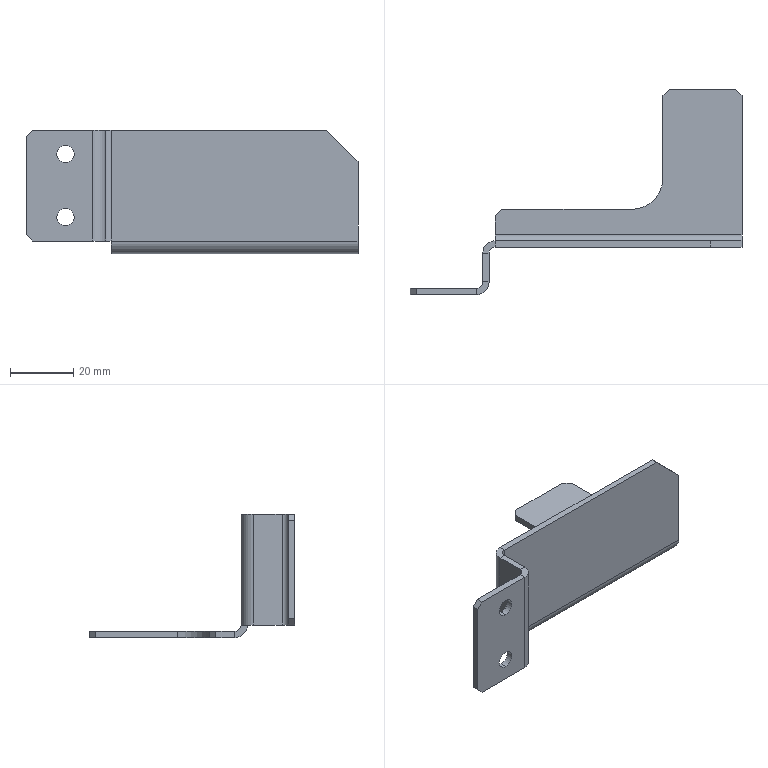Part | NX | features BREP 1 | 1 solid | 43 faces | box 105 x 65 x 39 mm | volume 11931 mm3 | plane 32 | cylinder 11 | commonest cylinder face diameters 5.5 x4 4 x3 8 x3 20 x1
STEP:
#1=CARTESIAN_POINT('',(2.,0.,17.5));
#2=VERTEX_POINT('',#1);
#3=CARTESIAN_POINT('',(0.,0.,15.5));
#4=VERTEX_POINT('',#3);
#5=CARTESIAN_POINT('',(0.,0.,15.5));
#6=DIRECTION('',(-0.7071,0.,-0.7071));
#7=VECTOR('',#6,1000.);
#8=LINE('',#5,#7);
#9=EDGE_CURVE('',#2,#4,#8,.T.);
#10=ORIENTED_EDGE('',*,*,#9,.F.);
#11=CARTESIAN_POINT('',(2.,2.,17.5));
#12=VERTEX_POINT('',#11);
#13=CARTESIAN_POINT('',(2.,4.,17.5));
#14=DIRECTION('',(0.,-1.,0.));
#15=VECTOR('',#14,1000.);
#16=LINE('',#13,#15);
#17=EDGE_CURVE('',#12,#2,#16,.T.);
#18=ORIENTED_EDGE('',*,*,#17,.F.);
#19=CARTESIAN_POINT('',(0.,2.,15.5));
#20=VERTEX_POINT('',#19);
#21=CARTESIAN_POINT('',(1.,2.,16.5));
#22=DIRECTION('',(0.7071,0.,0.7071));
#23=VECTOR('',#22,1000.);
#24=LINE('',#21,#23);
#25=EDGE_CURVE('',#20,#12,#24,.T.);
#26=ORIENTED_EDGE('',*,*,#25,.F.);
#27=CARTESIAN_POINT('',(0.,0.,15.5));
#28=DIRECTION('',(0.,1.,0.));
#29=VECTOR('',#28,1000.);
#30=LINE('',#27,#29);
#31=EDGE_CURVE('',#4,#20,#30,.T.);
#32=ORIENTED_EDGE('',*,*,#31,.F.);
#33=EDGE_LOOP('',(#10,#18,#26,#32));
#34=FACE_BOUND('',#33,.T.);
#35=CARTESIAN_POINT('',(0.,0.,15.5));
#36=DIRECTION('',(0.7071,0.,-0.7071));
#37=DIRECTION('',(0.,1.,0.));
#38=AXIS2_PLACEMENT_3D('',#35,#36,#37);
#39=PLANE('',#38);
#40=ADVANCED_FACE('',(#34),#39,.F.);
#41=CARTESIAN_POINT('',(0.,0.,-15.5));
#42=VERTEX_POINT('',#41);
#43=CARTESIAN_POINT('',(2.,0.,-17.5));
#44=VERTEX_POINT('',#43);
#45=CARTESIAN_POINT('',(2.,0.,-17.5));
#46=DIRECTION('',(0.7071,0.,-0.7071));
#47=VECTOR('',#46,1000.);
#48=LINE('',#45,#47);
#49=EDGE_CURVE('',#42,#44,#48,.T.);
#50=ORIENTED_EDGE('',*,*,#49,.F.);
#51=CARTESIAN_POINT('',(0.,2.,-15.5));
#52=VERTEX_POINT('',#51);
#53=CARTESIAN_POINT('',(0.,0.,-15.5));
#54=DIRECTION('',(0.,-1.,0.));
#55=VECTOR('',#54,1000.);
#56=LINE('',#53,#55);
#57=EDGE_CURVE('',#52,#42,#56,.T.);
#58=ORIENTED_EDGE('',*,*,#57,.F.);
#59=CARTESIAN_POINT('',(2.,2.,-17.5));
#60=VERTEX_POINT('',#59);
#61=CARTESIAN_POINT('',(-16.5,2.,1.));
#62=DIRECTION('',(-0.7071,0.,0.7071));
#63=VECTOR('',#62,1000.);
#64=LINE('',#61,#63);
#65=EDGE_CURVE('',#60,#52,#64,.T.);
#66=ORIENTED_EDGE('',*,*,#65,.F.);
#67=CARTESIAN_POINT('',(2.,2.,-17.5));
#68=DIRECTION('',(0.,1.,0.));
#69=VECTOR('',#68,1000.);
#70=LINE('',#67,#69);
#71=EDGE_CURVE('',#44,#60,#70,.T.);
#72=ORIENTED_EDGE('',*,*,#71,.F.);
#73=EDGE_LOOP('',(#50,#58,#66,#72));
#74=FACE_BOUND('',#73,.T.);
#75=CARTESIAN_POINT('',(2.,13.,-17.5));
#76=DIRECTION('',(-0.7071,0.,-0.7071));
#77=DIRECTION('',(0.,-1.,0.));
#78=AXIS2_PLACEMENT_3D('',#75,#76,#77);
#79=PLANE('',#78);
#80=ADVANCED_FACE('',(#74),#79,.T.);
#81=CARTESIAN_POINT('',(29.,27.,-19.5));
#82=VERTEX_POINT('',#81);
#83=CARTESIAN_POINT('',(27.,25.,-19.5));
#84=VERTEX_POINT('',#83);
#85=CARTESIAN_POINT('',(27.,25.,-19.5));
#86=DIRECTION('',(-0.7071,-0.7071,0.));
#87=VECTOR('',#86,1000.);
#88=LINE('',#85,#87);
#89=EDGE_CURVE('',#82,#84,#88,.T.);
#90=ORIENTED_EDGE('',*,*,#89,.F.);
#91=CARTESIAN_POINT('',(29.,27.,-21.5));
#92=VERTEX_POINT('',#91);
#93=CARTESIAN_POINT('',(29.,27.,-19.5));
#94=DIRECTION('',(0.,0.,1.));
#95=VECTOR('',#94,1000.);
#96=LINE('',#93,#95);
#97=EDGE_CURVE('',#92,#82,#96,.T.);
#98=ORIENTED_EDGE('',*,*,#97,.F.);
#99=CARTESIAN_POINT('',(27.,25.,-21.5));
#100=VERTEX_POINT('',#99);
#101=CARTESIAN_POINT('',(1.,-1.,-21.5));
#102=DIRECTION('',(0.7071,0.7071,0.));
#103=VECTOR('',#102,1000.);
#104=LINE('',#101,#103);
#105=EDGE_CURVE('',#100,#92,#104,.T.);
#106=ORIENTED_EDGE('',*,*,#105,.F.);
#107=CARTESIAN_POINT('',(27.,25.,-21.5));
#108=DIRECTION('',(0.,0.,-1.));
#109=VECTOR('',#108,1000.);
#110=LINE('',#107,#109);
#111=EDGE_CURVE('',#84,#100,#110,.T.);
#112=ORIENTED_EDGE('',*,*,#111,.F.);
#113=EDGE_LOOP('',(#90,#98,#106,#112));
#114=FACE_BOUND('',#113,.T.);
#115=CARTESIAN_POINT('',(27.,25.,-21.5));
#116=DIRECTION('',(-0.7071,0.7071,0.));
#117=DIRECTION('',(0.,0.,1.));
#118=AXIS2_PLACEMENT_3D('',#115,#116,#117);
#119=PLANE('',#118);
#120=ADVANCED_FACE('',(#114),#119,.T.);
#121=CARTESIAN_POINT('',(82.,65.,-19.5));
#122=VERTEX_POINT('',#121);
#123=CARTESIAN_POINT('',(80.,63.,-19.5));
#124=VERTEX_POINT('',#123);
#125=CARTESIAN_POINT('',(80.,63.,-19.5));
#126=DIRECTION('',(-0.7071,-0.7071,0.));
#127=VECTOR('',#126,1000.);
#128=LINE('',#125,#127);
#129=EDGE_CURVE('',#122,#124,#128,.T.);
#130=ORIENTED_EDGE('',*,*,#129,.F.);
#131=CARTESIAN_POINT('',(82.,65.,-21.5));
#132=VERTEX_POINT('',#131);
#133=CARTESIAN_POINT('',(82.,65.,-19.5));
#134=DIRECTION('',(0.,0.,1.));
#135=VECTOR('',#134,1000.);
#136=LINE('',#133,#135);
#137=EDGE_CURVE('',#132,#122,#136,.T.);
#138=ORIENTED_EDGE('',*,*,#137,.F.);
#139=CARTESIAN_POINT('',(80.,63.,-21.5));
#140=VERTEX_POINT('',#139);
#141=CARTESIAN_POINT('',(8.5,-8.5,-21.5));
#142=DIRECTION('',(0.7071,0.7071,0.));
#143=VECTOR('',#142,1000.);
#144=LINE('',#141,#143);
#145=EDGE_CURVE('',#140,#132,#144,.T.);
#146=ORIENTED_EDGE('',*,*,#145,.F.);
#147=CARTESIAN_POINT('',(80.,63.,-21.5));
#148=DIRECTION('',(0.,0.,-1.));
#149=VECTOR('',#148,1000.);
#150=LINE('',#147,#149);
#151=EDGE_CURVE('',#124,#140,#150,.T.);
#152=ORIENTED_EDGE('',*,*,#151,.F.);
#153=EDGE_LOOP('',(#130,#138,#146,#152));
#154=FACE_BOUND('',#153,.T.);
#155=CARTESIAN_POINT('',(80.,63.,17.5));
#156=DIRECTION('',(-0.7071,0.7071,0.));
#157=DIRECTION('',(0.,0.,1.));
#158=AXIS2_PLACEMENT_3D('',#155,#156,#157);
#159=PLANE('',#158);
#160=ADVANCED_FACE('',(#154),#159,.T.);
#161=CARTESIAN_POINT('',(103.,65.,-21.5));
#162=VERTEX_POINT('',#161);
#163=CARTESIAN_POINT('',(105.,63.,-21.5));
#164=VERTEX_POINT('',#163);
#165=CARTESIAN_POINT('',(84.,84.,-21.5));
#166=DIRECTION('',(0.7071,-0.7071,0.));
#167=VECTOR('',#166,1000.);
#168=LINE('',#165,#167);
#169=EDGE_CURVE('',#162,#164,#168,.T.);
#170=ORIENTED_EDGE('',*,*,#169,.F.);
#171=CARTESIAN_POINT('',(103.,65.,-19.5));
#172=VERTEX_POINT('',#171);
#173=CARTESIAN_POINT('',(103.,65.,-21.5));
#174=DIRECTION('',(0.,0.,-1.));
#175=VECTOR('',#174,1000.);
#176=LINE('',#173,#175);
#177=EDGE_CURVE('',#172,#162,#176,.T.);
#178=ORIENTED_EDGE('',*,*,#177,.F.);
#179=CARTESIAN_POINT('',(105.,63.,-19.5));
#180=VERTEX_POINT('',#179);
#181=CARTESIAN_POINT('',(105.,63.,-19.5));
#182=DIRECTION('',(-0.7071,0.7071,0.));
#183=VECTOR('',#182,1000.);
#184=LINE('',#181,#183);
#185=EDGE_CURVE('',#180,#172,#184,.T.);
#186=ORIENTED_EDGE('',*,*,#185,.F.);
#187=CARTESIAN_POINT('',(105.,63.,-21.5));
#188=DIRECTION('',(0.,0.,1.));
#189=VECTOR('',#188,1000.);
#190=LINE('',#187,#189);
#191=EDGE_CURVE('',#164,#180,#190,.T.);
#192=ORIENTED_EDGE('',*,*,#191,.F.);
#193=EDGE_LOOP('',(#170,#178,#186,#192));
#194=FACE_BOUND('',#193,.T.);
#195=CARTESIAN_POINT('',(105.,63.,-21.5));
#196=DIRECTION('',(-0.7071,-0.7071,0.));
#197=DIRECTION('',(0.,0.,1.));
#198=AXIS2_PLACEMENT_3D('',#195,#196,#197);
#199=PLANE('',#198);
#200=ADVANCED_FACE('',(#194),#199,.F.);
#201=CARTESIAN_POINT('',(80.,37.,-19.5));
#202=VERTEX_POINT('',#201);
#203=CARTESIAN_POINT('',(70.,27.,-19.5));
#204=VERTEX_POINT('',#203);
#205=CARTESIAN_POINT('',(70.,37.,-19.5));
#206=DIRECTION('',(0.,0.,-1.));
#207=DIRECTION('',(-1.,0.,0.));
#208=AXIS2_PLACEMENT_3D('',#205,#206,#207);
#209=CIRCLE('',#208,10.);
#210=EDGE_CURVE('',#202,#204,#209,.T.);
#211=ORIENTED_EDGE('',*,*,#210,.F.);
#212=CARTESIAN_POINT('',(80.,37.,-21.5));
#213=VERTEX_POINT('',#212);
#214=CARTESIAN_POINT('',(80.,37.,-19.5));
#215=DIRECTION('',(0.,0.,1.));
#216=VECTOR('',#215,1000.);
#217=LINE('',#214,#216);
#218=EDGE_CURVE('',#213,#202,#217,.T.);
#219=ORIENTED_EDGE('',*,*,#218,.F.);
#220=CARTESIAN_POINT('',(70.,27.,-21.5));
#221=VERTEX_POINT('',#220);
#222=CARTESIAN_POINT('',(70.,37.,-21.5));
#223=DIRECTION('',(0.,0.,1.));
#224=DIRECTION('',(-1.,0.,0.));
#225=AXIS2_PLACEMENT_3D('',#222,#223,#224);
#226=CIRCLE('',#225,10.);
#227=EDGE_CURVE('',#221,#213,#226,.T.);
#228=ORIENTED_EDGE('',*,*,#227,.F.);
#229=CARTESIAN_POINT('',(70.,27.,-21.5));
#230=DIRECTION('',(0.,0.,-1.));
#231=VECTOR('',#230,1000.);
#232=LINE('',#229,#231);
#233=EDGE_CURVE('',#204,#221,#232,.T.);
#234=ORIENTED_EDGE('',*,*,#233,.F.);
#235=EDGE_LOOP('',(#211,#219,#228,#234));
#236=FACE_BOUND('',#235,.T.);
#237=CARTESIAN_POINT('',(70.,37.,17.5));
#238=DIRECTION('',(0.,0.,1.));
#239=DIRECTION('',(1.,0.,0.));
#240=AXIS2_PLACEMENT_3D('',#237,#238,#239);
#241=CYLINDRICAL_SURFACE('',#240,10.);
#242=ADVANCED_FACE('',(#236),#241,.F.);
#243=CARTESIAN_POINT('',(95.,17.,17.5));
#244=VERTEX_POINT('',#243);
#245=CARTESIAN_POINT('',(105.,17.,7.5));
#246=VERTEX_POINT('',#245);
#247=CARTESIAN_POINT('',(60.,17.,52.5));
#248=DIRECTION('',(0.7071,0.,-0.7071));
#249=VECTOR('',#248,1000.);
#250=LINE('',#247,#249);
#251=EDGE_CURVE('',#244,#246,#250,.T.);
#252=ORIENTED_EDGE('',*,*,#251,.F.);
#253=CARTESIAN_POINT('',(95.,15.,17.5));
#254=VERTEX_POINT('',#253);
#255=CARTESIAN_POINT('',(95.,13.,17.5));
#256=DIRECTION('',(0.,1.,0.));
#257=VECTOR('',#256,1000.);
#258=LINE('',#255,#257);
#259=EDGE_CURVE('',#254,#244,#258,.T.);
#260=ORIENTED_EDGE('',*,*,#259,.F.);
#261=CARTESIAN_POINT('',(105.,15.,7.5));
#262=VERTEX_POINT('',#261);
#263=CARTESIAN_POINT('',(105.,15.,7.5));
#264=DIRECTION('',(-0.7071,0.,0.7071));
#265=VECTOR('',#264,1000.);
#266=LINE('',#263,#265);
#267=EDGE_CURVE('',#262,#254,#266,.T.);
#268=ORIENTED_EDGE('',*,*,#267,.F.);
#269=CARTESIAN_POINT('',(105.,17.,7.5));
#270=DIRECTION('',(0.,-1.,0.));
#271=VECTOR('',#270,1000.);
#272=LINE('',#269,#271);
#273=EDGE_CURVE('',#246,#262,#272,.T.);
#274=ORIENTED_EDGE('',*,*,#273,.F.);
#275=EDGE_LOOP('',(#252,#260,#268,#274));
#276=FACE_BOUND('',#275,.T.);
#277=CARTESIAN_POINT('',(105.,17.,7.5));
#278=DIRECTION('',(-0.7071,0.,-0.7071));
#279=DIRECTION('',(0.,-1.,0.));
#280=AXIS2_PLACEMENT_3D('',#277,#278,#279);
#281=PLANE('',#280);
#282=ADVANCED_FACE('',(#276),#281,.F.);
#283=CARTESIAN_POINT('',(12.5,2.,-12.75));
#284=VERTEX_POINT('',#283);
#285=CARTESIAN_POINT('',(12.5,0.,-12.75));
#286=VERTEX_POINT('',#285);
#287=CARTESIAN_POINT('',(12.5,2.,-12.75));
#288=DIRECTION('',(0.,1.,0.));
#289=VECTOR('',#288,1000.);
#290=LINE('',#287,#289);
#291=EDGE_CURVE('',#284,#286,#290,.F.);
#292=ORIENTED_EDGE('',*,*,#291,.T.);
#293=CARTESIAN_POINT('',(12.5,0.,-7.25));
#294=VERTEX_POINT('',#293);
#295=CARTESIAN_POINT('',(12.5,0.,-10.));
#296=DIRECTION('',(0.,1.,0.));
#297=DIRECTION('',(0.,0.,1.));
#298=AXIS2_PLACEMENT_3D('',#295,#296,#297);
#299=CIRCLE('',#298,2.75);
#300=EDGE_CURVE('',#294,#286,#299,.T.);
#301=ORIENTED_EDGE('',*,*,#300,.F.);
#302=CARTESIAN_POINT('',(12.5,2.,-7.25));
#303=VERTEX_POINT('',#302);
#304=CARTESIAN_POINT('',(12.5,2.,-7.25));
#305=DIRECTION('',(0.,1.,0.));
#306=VECTOR('',#305,1000.);
#307=LINE('',#304,#306);
#308=EDGE_CURVE('',#303,#294,#307,.F.);
#309=ORIENTED_EDGE('',*,*,#308,.F.);
#310=CARTESIAN_POINT('',(12.5,2.,-10.));
#311=DIRECTION('',(0.,1.,0.));
#312=DIRECTION('',(0.,0.,1.));
#313=AXIS2_PLACEMENT_3D('',#310,#311,#312);
#314=CIRCLE('',#313,2.75);
#315=EDGE_CURVE('',#303,#284,#314,.T.);
#316=ORIENTED_EDGE('',*,*,#315,.T.);
#317=EDGE_LOOP('',(#292,#301,#309,#316));
#318=FACE_BOUND('',#317,.T.);
#319=CARTESIAN_POINT('',(12.5,2.,-10.));
#320=DIRECTION('',(0.,1.,0.));
#321=DIRECTION('',(0.,0.,1.));
#322=AXIS2_PLACEMENT_3D('',#319,#320,#321);
#323=CYLINDRICAL_SURFACE('',#322,2.75);
#324=ADVANCED_FACE('',(#318),#323,.F.);
#325=CARTESIAN_POINT('',(12.5,2.,7.25));
#326=VERTEX_POINT('',#325);
#327=CARTESIAN_POINT('',(12.5,0.,7.25));
#328=VERTEX_POINT('',#327);
#329=CARTESIAN_POINT('',(12.5,2.,7.25));
#330=DIRECTION('',(0.,1.,0.));
#331=VECTOR('',#330,1000.);
#332=LINE('',#329,#331);
#333=EDGE_CURVE('',#326,#328,#332,.F.);
#334=ORIENTED_EDGE('',*,*,#333,.T.);
#335=CARTESIAN_POINT('',(12.5,0.,12.75));
#336=VERTEX_POINT('',#335);
#337=CARTESIAN_POINT('',(12.5,0.,10.));
#338=DIRECTION('',(0.,1.,0.));
#339=DIRECTION('',(0.,0.,1.));
#340=AXIS2_PLACEMENT_3D('',#337,#338,#339);
#341=CIRCLE('',#340,2.75);
#342=EDGE_CURVE('',#336,#328,#341,.T.);
#343=ORIENTED_EDGE('',*,*,#342,.F.);
#344=CARTESIAN_POINT('',(12.5,2.,12.75));
#345=VERTEX_POINT('',#344);
#346=CARTESIAN_POINT('',(12.5,2.,12.75));
#347=DIRECTION('',(0.,1.,0.));
#348=VECTOR('',#347,1000.);
#349=LINE('',#346,#348);
#350=EDGE_CURVE('',#345,#336,#349,.F.);
#351=ORIENTED_EDGE('',*,*,#350,.F.);
#352=CARTESIAN_POINT('',(12.5,2.,10.));
#353=DIRECTION('',(0.,1.,0.));
#354=DIRECTION('',(0.,0.,1.));
#355=AXIS2_PLACEMENT_3D('',#352,#353,#354);
#356=CIRCLE('',#355,2.75);
#357=EDGE_CURVE('',#345,#326,#356,.T.);
#358=ORIENTED_EDGE('',*,*,#357,.T.);
#359=EDGE_LOOP('',(#334,#343,#351,#358));
#360=FACE_BOUND('',#359,.T.);
#361=CARTESIAN_POINT('',(12.5,2.,10.));
#362=DIRECTION('',(0.,1.,0.));
#363=DIRECTION('',(0.,0.,1.));
#364=AXIS2_PLACEMENT_3D('',#361,#362,#363);
#365=CYLINDRICAL_SURFACE('',#364,2.75);
#366=ADVANCED_FACE('',(#360),#365,.F.);
#367=CARTESIAN_POINT('',(80.,0.,-19.5));
#368=DIRECTION('',(0.,-1.,0.));
#369=VECTOR('',#368,1000.);
#370=LINE('',#367,#369);
#371=EDGE_CURVE('',#124,#202,#370,.T.);
#372=ORIENTED_EDGE('',*,*,#371,.F.);
#373=ORIENTED_EDGE('',*,*,#151,.T.);
#374=CARTESIAN_POINT('',(80.,65.,-21.5));
#375=DIRECTION('',(0.,-1.,0.));
#376=VECTOR('',#375,1000.);
#377=LINE('',#374,#376);
#378=EDGE_CURVE('',#140,#213,#377,.T.);
#379=ORIENTED_EDGE('',*,*,#378,.T.);
#380=ORIENTED_EDGE('',*,*,#218,.T.);
#381=EDGE_LOOP('',(#372,#373,#379,#380));
#382=FACE_BOUND('',#381,.T.);
#383=CARTESIAN_POINT('',(80.,65.,17.5));
#384=DIRECTION('',(1.,0.,0.));
#385=DIRECTION('',(0.,0.,-1.));
#386=AXIS2_PLACEMENT_3D('',#383,#384,#385);
#387=PLANE('',#386);
#388=ADVANCED_FACE('',(#382),#387,.F.);
#389=CARTESIAN_POINT('',(27.,27.,-21.5));
#390=DIRECTION('',(-1.,0.,0.));
#391=VECTOR('',#390,1000.);
#392=LINE('',#389,#391);
#393=EDGE_CURVE('',#221,#92,#392,.T.);
#394=ORIENTED_EDGE('',*,*,#393,.T.);
#395=ORIENTED_EDGE('',*,*,#97,.T.);
#396=CARTESIAN_POINT('',(0.,27.,-19.5));
#397=DIRECTION('',(-1.,0.,0.));
#398=VECTOR('',#397,1000.);
#399=LINE('',#396,#398);
#400=EDGE_CURVE('',#204,#82,#399,.T.);
#401=ORIENTED_EDGE('',*,*,#400,.F.);
#402=ORIENTED_EDGE('',*,*,#233,.T.);
#403=EDGE_LOOP('',(#394,#395,#401,#402));
#404=FACE_BOUND('',#403,.T.);
#405=CARTESIAN_POINT('',(27.,27.,17.5));
#406=DIRECTION('',(0.,-1.,0.));
#407=DIRECTION('',(1.,0.,0.));
#408=AXIS2_PLACEMENT_3D('',#405,#406,#407);
#409=PLANE('',#408);
#410=ADVANCED_FACE('',(#404),#409,.F.);
#411=CARTESIAN_POINT('',(0.,65.,-19.5));
#412=DIRECTION('',(-1.,0.,0.));
#413=VECTOR('',#412,1000.);
#414=LINE('',#411,#413);
#415=EDGE_CURVE('',#172,#122,#414,.T.);
#416=ORIENTED_EDGE('',*,*,#415,.F.);
#417=ORIENTED_EDGE('',*,*,#177,.T.);
#418=CARTESIAN_POINT('',(27.,65.,-21.5));
#419=DIRECTION('',(-1.,0.,0.));
#420=VECTOR('',#419,1000.);
#421=LINE('',#418,#420);
#422=EDGE_CURVE('',#162,#132,#421,.T.);
#423=ORIENTED_EDGE('',*,*,#422,.T.);
#424=ORIENTED_EDGE('',*,*,#137,.T.);
#425=EDGE_LOOP('',(#416,#417,#423,#424));
#426=FACE_BOUND('',#425,.T.);
#427=CARTESIAN_POINT('',(27.,65.,-21.5));
#428=DIRECTION('',(0.,1.,0.));
#429=DIRECTION('',(0.,0.,1.));
#430=AXIS2_PLACEMENT_3D('',#427,#428,#429);
#431=PLANE('',#430);
#432=ADVANCED_FACE('',(#426),#431,.T.);
#433=CARTESIAN_POINT('',(105.,19.,-19.5));
#434=VERTEX_POINT('',#433);
#435=CARTESIAN_POINT('',(105.,0.,-19.5));
#436=DIRECTION('',(0.,1.,0.));
#437=VECTOR('',#436,1000.);
#438=LINE('',#435,#437);
#439=EDGE_CURVE('',#434,#180,#438,.T.);
#440=ORIENTED_EDGE('',*,*,#439,.T.);
#441=ORIENTED_EDGE('',*,*,#185,.T.);
#442=ORIENTED_EDGE('',*,*,#415,.T.);
#443=ORIENTED_EDGE('',*,*,#129,.T.);
#444=ORIENTED_EDGE('',*,*,#371,.T.);
#445=ORIENTED_EDGE('',*,*,#210,.T.);
#446=ORIENTED_EDGE('',*,*,#400,.T.);
#447=ORIENTED_EDGE('',*,*,#89,.T.);
#448=CARTESIAN_POINT('',(27.,19.,-19.5));
#449=VERTEX_POINT('',#448);
#450=CARTESIAN_POINT('',(27.,0.,-19.5));
#451=DIRECTION('',(0.,-1.,0.));
#452=VECTOR('',#451,1000.);
#453=LINE('',#450,#452);
#454=EDGE_CURVE('',#84,#449,#453,.T.);
#455=ORIENTED_EDGE('',*,*,#454,.T.);
#456=CARTESIAN_POINT('',(105.,19.,-19.5));
#457=DIRECTION('',(-1.,0.,0.));
#458=VECTOR('',#457,1000.);
#459=LINE('',#456,#458);
#460=EDGE_CURVE('',#434,#449,#459,.T.);
#461=ORIENTED_EDGE('',*,*,#460,.F.);
#462=EDGE_LOOP('',(#440,#441,#442,#443,#444,#445,#446,#447,#455,#461));
#463=FACE_BOUND('',#462,.T.);
#464=CARTESIAN_POINT('',(0.,0.,-19.5));
#465=DIRECTION('',(0.,0.,-1.));
#466=DIRECTION('',(-1.,0.,0.));
#467=AXIS2_PLACEMENT_3D('',#464,#465,#466);
#468=PLANE('',#467);
#469=ADVANCED_FACE('',(#463),#468,.F.);
#470=ORIENTED_EDGE('',*,*,#422,.F.);
#471=ORIENTED_EDGE('',*,*,#169,.T.);
#472=CARTESIAN_POINT('',(105.,19.,-21.5));
#473=VERTEX_POINT('',#472);
#474=CARTESIAN_POINT('',(105.,65.,-21.5));
#475=DIRECTION('',(0.,1.,0.));
#476=VECTOR('',#475,1000.);
#477=LINE('',#474,#476);
#478=EDGE_CURVE('',#473,#164,#477,.T.);
#479=ORIENTED_EDGE('',*,*,#478,.F.);
#480=CARTESIAN_POINT('',(27.,19.,-21.5));
#481=VERTEX_POINT('',#480);
#482=CARTESIAN_POINT('',(0.,19.,-21.5));
#483=DIRECTION('',(-1.,0.,0.));
#484=VECTOR('',#483,1000.);
#485=LINE('',#482,#484);
#486=EDGE_CURVE('',#473,#481,#485,.T.);
#487=ORIENTED_EDGE('',*,*,#486,.T.);
#488=CARTESIAN_POINT('',(27.,17.,-21.5));
#489=DIRECTION('',(0.,-1.,0.));
#490=VECTOR('',#489,1000.);
#491=LINE('',#488,#490);
#492=EDGE_CURVE('',#100,#481,#491,.T.);
#493=ORIENTED_EDGE('',*,*,#492,.F.);
#494=ORIENTED_EDGE('',*,*,#105,.T.);
#495=ORIENTED_EDGE('',*,*,#393,.F.);
#496=ORIENTED_EDGE('',*,*,#227,.T.);
#497=ORIENTED_EDGE('',*,*,#378,.F.);
#498=ORIENTED_EDGE('',*,*,#145,.T.);
#499=EDGE_LOOP('',(#470,#471,#479,#487,#493,#494,#495,#496,#497,#498));
#500=FACE_BOUND('',#499,.T.);
#501=CARTESIAN_POINT('',(0.,0.,-21.5));
#502=DIRECTION('',(0.,0.,-1.));
#503=DIRECTION('',(-1.,0.,0.));
#504=AXIS2_PLACEMENT_3D('',#501,#502,#503);
#505=PLANE('',#504);
#506=ADVANCED_FACE('',(#500),#505,.T.);
#507=ORIENTED_EDGE('',*,*,#478,.T.);
#508=ORIENTED_EDGE('',*,*,#191,.T.);
#509=ORIENTED_EDGE('',*,*,#439,.F.);
#510=CARTESIAN_POINT('',(105.,19.,-21.5));
#511=DIRECTION('',(0.,0.,-1.));
#512=VECTOR('',#511,1000.);
#513=LINE('',#510,#512);
#514=EDGE_CURVE('',#434,#473,#513,.T.);
#515=ORIENTED_EDGE('',*,*,#514,.T.);
#516=EDGE_LOOP('',(#507,#508,#509,#515));
#517=FACE_BOUND('',#516,.T.);
#518=CARTESIAN_POINT('',(105.,65.,-21.5));
#519=DIRECTION('',(1.,0.,0.));
#520=DIRECTION('',(0.,0.,-1.));
#521=AXIS2_PLACEMENT_3D('',#518,#519,#520);
#522=PLANE('',#521);
#523=ADVANCED_FACE('',(#517),#522,.T.);
#524=ORIENTED_EDGE('',*,*,#454,.F.);
#525=ORIENTED_EDGE('',*,*,#111,.T.);
#526=ORIENTED_EDGE('',*,*,#492,.T.);
#527=CARTESIAN_POINT('',(27.,19.,-19.5));
#528=DIRECTION('',(0.,0.,-1.));
#529=VECTOR('',#528,1000.);
#530=LINE('',#527,#529);
#531=EDGE_CURVE('',#449,#481,#530,.T.);
#532=ORIENTED_EDGE('',*,*,#531,.F.);
#533=EDGE_LOOP('',(#524,#525,#526,#532));
#534=FACE_BOUND('',#533,.T.);
#535=CARTESIAN_POINT('',(27.,17.,-21.5));
#536=DIRECTION('',(-1.,0.,0.));
#537=DIRECTION('',(0.,0.,1.));
#538=AXIS2_PLACEMENT_3D('',#535,#536,#537);
#539=PLANE('',#538);
#540=ADVANCED_FACE('',(#534),#539,.T.);
#541=CARTESIAN_POINT('',(27.,17.,-17.5));
#542=VERTEX_POINT('',#541);
#543=CARTESIAN_POINT('',(105.,17.,-17.5));
#544=VERTEX_POINT('',#543);
#545=CARTESIAN_POINT('',(25.,17.,-17.5));
#546=DIRECTION('',(1.,0.,0.));
#547=VECTOR('',#546,1000.);
#548=LINE('',#545,#547);
#549=EDGE_CURVE('',#542,#544,#548,.T.);
#550=ORIENTED_EDGE('',*,*,#549,.T.);
#551=CARTESIAN_POINT('',(105.,19.,-17.5));
#552=DIRECTION('',(1.,0.,0.));
#553=DIRECTION('',(0.,0.,1.));
#554=AXIS2_PLACEMENT_3D('',#551,#552,#553);
#555=CIRCLE('',#554,2.);
#556=EDGE_CURVE('',#544,#434,#555,.T.);
#557=ORIENTED_EDGE('',*,*,#556,.T.);
#558=ORIENTED_EDGE('',*,*,#460,.T.);
#559=CARTESIAN_POINT('',(27.,19.,-17.5));
#560=DIRECTION('',(-1.,0.,0.));
#561=DIRECTION('',(0.,0.,1.));
#562=AXIS2_PLACEMENT_3D('',#559,#560,#561);
#563=CIRCLE('',#562,2.);
#564=EDGE_CURVE('',#449,#542,#563,.T.);
#565=ORIENTED_EDGE('',*,*,#564,.T.);
#566=EDGE_LOOP('',(#550,#557,#558,#565));
#567=FACE_BOUND('',#566,.T.);
#568=CARTESIAN_POINT('',(27.,19.,-17.5));
#569=DIRECTION('',(-1.,0.,0.));
#570=DIRECTION('',(0.,0.,-1.));
#571=AXIS2_PLACEMENT_3D('',#568,#569,#570);
#572=CYLINDRICAL_SURFACE('',#571,2.);
#573=ADVANCED_FACE('',(#567),#572,.F.);
#574=CARTESIAN_POINT('',(27.,15.,-17.5));
#575=VERTEX_POINT('',#574);
#576=CARTESIAN_POINT('',(105.,15.,-17.5));
#577=VERTEX_POINT('',#576);
#578=CARTESIAN_POINT('',(25.,15.,-17.5));
#579=DIRECTION('',(1.,0.,0.));
#580=VECTOR('',#579,1000.);
#581=LINE('',#578,#580);
#582=EDGE_CURVE('',#575,#577,#581,.T.);
#583=ORIENTED_EDGE('',*,*,#582,.F.);
#584=CARTESIAN_POINT('',(27.,19.,-17.5));
#585=DIRECTION('',(-1.,0.,0.));
#586=DIRECTION('',(0.,0.,1.));
#587=AXIS2_PLACEMENT_3D('',#584,#585,#586);
#588=CIRCLE('',#587,4.);
#589=EDGE_CURVE('',#481,#575,#588,.T.);
#590=ORIENTED_EDGE('',*,*,#589,.F.);
#591=ORIENTED_EDGE('',*,*,#486,.F.);
#592=CARTESIAN_POINT('',(105.,19.,-17.5));
#593=DIRECTION('',(1.,0.,0.));
#594=DIRECTION('',(0.,0.,1.));
#595=AXIS2_PLACEMENT_3D('',#592,#593,#594);
#596=CIRCLE('',#595,4.);
#597=EDGE_CURVE('',#577,#473,#596,.T.);
#598=ORIENTED_EDGE('',*,*,#597,.F.);
#599=EDGE_LOOP('',(#583,#590,#591,#598));
#600=FACE_BOUND('',#599,.T.);
#601=CARTESIAN_POINT('',(27.,19.,-17.5));
#602=DIRECTION('',(-1.,0.,0.));
#603=DIRECTION('',(0.,0.,-1.));
#604=AXIS2_PLACEMENT_3D('',#601,#602,#603);
#605=CYLINDRICAL_SURFACE('',#604,4.);
#606=ADVANCED_FACE('',(#600),#605,.T.);
#607=ORIENTED_EDGE('',*,*,#564,.F.);
#608=ORIENTED_EDGE('',*,*,#531,.T.);
#609=ORIENTED_EDGE('',*,*,#589,.T.);
#610=CARTESIAN_POINT('',(27.,15.,-17.5));
#611=DIRECTION('',(0.,1.,0.));
#612=VECTOR('',#611,1000.);
#613=LINE('',#610,#612);
#614=EDGE_CURVE('',#575,#542,#613,.T.);
#615=ORIENTED_EDGE('',*,*,#614,.T.);
#616=EDGE_LOOP('',(#607,#608,#609,#615));
#617=FACE_BOUND('',#616,.T.);
#618=CARTESIAN_POINT('',(27.,19.,-17.5));
#619=DIRECTION('',(1.,0.,0.));
#620=DIRECTION('',(0.,0.,-1.));
#621=AXIS2_PLACEMENT_3D('',#618,#619,#620);
#622=PLANE('',#621);
#623=ADVANCED_FACE('',(#617),#622,.F.);
#624=ORIENTED_EDGE('',*,*,#514,.F.);
#625=ORIENTED_EDGE('',*,*,#556,.F.);
#626=CARTESIAN_POINT('',(105.,17.,-17.5));
#627=DIRECTION('',(0.,-1.,0.));
#628=VECTOR('',#627,1000.);
#629=LINE('',#626,#628);
#630=EDGE_CURVE('',#544,#577,#629,.T.);
#631=ORIENTED_EDGE('',*,*,#630,.T.);
#632=ORIENTED_EDGE('',*,*,#597,.T.);
#633=EDGE_LOOP('',(#624,#625,#631,#632));
#634=FACE_BOUND('',#633,.T.);
#635=CARTESIAN_POINT('',(105.,19.,-17.5));
#636=DIRECTION('',(1.,0.,0.));
#637=DIRECTION('',(0.,0.,-1.));
#638=AXIS2_PLACEMENT_3D('',#635,#636,#637);
#639=PLANE('',#638);
#640=ADVANCED_FACE('',(#634),#639,.T.);
#641=CARTESIAN_POINT('',(21.,0.,-17.5));
#642=VERTEX_POINT('',#641);
#643=CARTESIAN_POINT('',(0.,0.,-17.5));
#644=DIRECTION('',(1.,0.,0.));
#645=VECTOR('',#644,1000.);
#646=LINE('',#643,#645);
#647=EDGE_CURVE('',#44,#642,#646,.T.);
#648=ORIENTED_EDGE('',*,*,#647,.F.);
#649=ORIENTED_EDGE('',*,*,#71,.T.);
#650=CARTESIAN_POINT('',(21.,2.,-17.5));
#651=VERTEX_POINT('',#650);
#652=CARTESIAN_POINT('',(0.,2.,-17.5));
#653=DIRECTION('',(1.,0.,0.));
#654=VECTOR('',#653,1000.);
#655=LINE('',#652,#654);
#656=EDGE_CURVE('',#60,#651,#655,.T.);
#657=ORIENTED_EDGE('',*,*,#656,.T.);
#658=CARTESIAN_POINT('',(21.,2.,-17.5));
#659=DIRECTION('',(0.,-1.,0.));
#660=VECTOR('',#659,1000.);
#661=LINE('',#658,#660);
#662=EDGE_CURVE('',#651,#642,#661,.T.);
#663=ORIENTED_EDGE('',*,*,#662,.T.);
#664=EDGE_LOOP('',(#648,#649,#657,#663));
#665=FACE_BOUND('',#664,.T.);
#666=CARTESIAN_POINT('',(27.,13.,-17.5));
#667=DIRECTION('',(0.,0.,1.));
#668=DIRECTION('',(1.,0.,0.));
#669=AXIS2_PLACEMENT_3D('',#666,#667,#668);
#670=PLANE('',#669);
#671=ADVANCED_FACE('',(#665),#670,.F.);
#672=CARTESIAN_POINT('',(27.,15.,17.5));
#673=VERTEX_POINT('',#672);
#674=CARTESIAN_POINT('',(25.,15.,17.5));
#675=DIRECTION('',(1.,0.,0.));
#676=VECTOR('',#675,1000.);
#677=LINE('',#674,#676);
#678=EDGE_CURVE('',#673,#254,#677,.T.);
#679=ORIENTED_EDGE('',*,*,#678,.T.);
#680=ORIENTED_EDGE('',*,*,#259,.T.);
#681=CARTESIAN_POINT('',(27.,17.,17.5));
#682=VERTEX_POINT('',#681);
#683=CARTESIAN_POINT('',(25.,17.,17.5));
#684=DIRECTION('',(1.,0.,0.));
#685=VECTOR('',#684,1000.);
#686=LINE('',#683,#685);
#687=EDGE_CURVE('',#682,#244,#686,.T.);
#688=ORIENTED_EDGE('',*,*,#687,.F.);
#689=CARTESIAN_POINT('',(27.,17.,17.5));
#690=DIRECTION('',(0.,-1.,0.));
#691=VECTOR('',#690,1000.);
#692=LINE('',#689,#691);
#693=EDGE_CURVE('',#682,#673,#692,.T.);
#694=ORIENTED_EDGE('',*,*,#693,.T.);
#695=EDGE_LOOP('',(#679,#680,#688,#694));
#696=FACE_BOUND('',#695,.T.);
#697=CARTESIAN_POINT('',(27.,13.,17.5));
#698=DIRECTION('',(0.,0.,1.));
#699=DIRECTION('',(1.,0.,0.));
#700=AXIS2_PLACEMENT_3D('',#697,#698,#699);
#701=PLANE('',#700);
#702=ADVANCED_FACE('',(#696),#701,.T.);
#703=CARTESIAN_POINT('',(25.,13.,-17.5));
#704=VERTEX_POINT('',#703);
#705=CARTESIAN_POINT('',(27.,13.,-17.5));
#706=DIRECTION('',(0.,0.,-1.));
#707=DIRECTION('',(1.,0.,0.));
#708=AXIS2_PLACEMENT_3D('',#705,#706,#707);
#709=CIRCLE('',#708,2.);
#710=EDGE_CURVE('',#704,#575,#709,.T.);
#711=ORIENTED_EDGE('',*,*,#710,.T.);
#712=CARTESIAN_POINT('',(27.,15.,17.5));
#713=DIRECTION('',(0.,0.,-1.));
#714=VECTOR('',#713,1000.);
#715=LINE('',#712,#714);
#716=EDGE_CURVE('',#673,#575,#715,.T.);
#717=ORIENTED_EDGE('',*,*,#716,.F.);
#718=CARTESIAN_POINT('',(25.,13.,17.5));
#719=VERTEX_POINT('',#718);
#720=CARTESIAN_POINT('',(27.,13.,17.5));
#721=DIRECTION('',(0.,0.,-1.));
#722=DIRECTION('',(1.,0.,0.));
#723=AXIS2_PLACEMENT_3D('',#720,#721,#722);
#724=CIRCLE('',#723,2.);
#725=EDGE_CURVE('',#719,#673,#724,.T.);
#726=ORIENTED_EDGE('',*,*,#725,.F.);
#727=CARTESIAN_POINT('',(25.,13.,17.5));
#728=DIRECTION('',(0.,0.,-1.));
#729=VECTOR('',#728,1000.);
#730=LINE('',#727,#729);
#731=EDGE_CURVE('',#719,#704,#730,.T.);
#732=ORIENTED_EDGE('',*,*,#731,.T.);
#733=EDGE_LOOP('',(#711,#717,#726,#732));
#734=FACE_BOUND('',#733,.T.);
#735=CARTESIAN_POINT('',(27.,13.,17.5));
#736=DIRECTION('',(0.,0.,-1.));
#737=DIRECTION('',(-1.,0.,0.));
#738=AXIS2_PLACEMENT_3D('',#735,#736,#737);
#739=CYLINDRICAL_SURFACE('',#738,2.);
#740=ADVANCED_FACE('',(#734),#739,.F.);
#741=CARTESIAN_POINT('',(25.,4.,-17.5));
#742=VERTEX_POINT('',#741);
#743=CARTESIAN_POINT('',(25.,0.,-17.5));
#744=DIRECTION('',(0.,1.,0.));
#745=VECTOR('',#744,1000.);
#746=LINE('',#743,#745);
#747=EDGE_CURVE('',#742,#704,#746,.T.);
#748=ORIENTED_EDGE('',*,*,#747,.T.);
#749=ORIENTED_EDGE('',*,*,#731,.F.);
#750=CARTESIAN_POINT('',(25.,4.,17.5));
#751=VERTEX_POINT('',#750);
#752=CARTESIAN_POINT('',(25.,0.,17.5));
#753=DIRECTION('',(0.,1.,0.));
#754=VECTOR('',#753,1000.);
#755=LINE('',#752,#754);
#756=EDGE_CURVE('',#751,#719,#755,.T.);
#757=ORIENTED_EDGE('',*,*,#756,.F.);
#758=CARTESIAN_POINT('',(25.,4.,17.5));
#759=DIRECTION('',(0.,0.,-1.));
#760=VECTOR('',#759,1000.);
#761=LINE('',#758,#760);
#762=EDGE_CURVE('',#751,#742,#761,.T.);
#763=ORIENTED_EDGE('',*,*,#762,.T.);
#764=EDGE_LOOP('',(#748,#749,#757,#763));
#765=FACE_BOUND('',#764,.T.);
#766=CARTESIAN_POINT('',(25.,0.,17.5));
#767=DIRECTION('',(-1.,0.,0.));
#768=DIRECTION('',(0.,0.,1.));
#769=AXIS2_PLACEMENT_3D('',#766,#767,#768);
#770=PLANE('',#769);
#771=ADVANCED_FACE('',(#765),#770,.F.);
#772=CARTESIAN_POINT('',(21.,4.,-17.5));
#773=DIRECTION('',(0.,0.,1.));
#774=DIRECTION('',(-1.,0.,0.));
#775=AXIS2_PLACEMENT_3D('',#772,#773,#774);
#776=CIRCLE('',#775,4.);
#777=EDGE_CURVE('',#642,#742,#776,.T.);
#778=ORIENTED_EDGE('',*,*,#777,.T.);
#779=ORIENTED_EDGE('',*,*,#762,.F.);
#780=CARTESIAN_POINT('',(21.,0.,17.5));
#781=VERTEX_POINT('',#780);
#782=CARTESIAN_POINT('',(21.,4.,17.5));
#783=DIRECTION('',(0.,0.,1.));
#784=DIRECTION('',(-1.,0.,0.));
#785=AXIS2_PLACEMENT_3D('',#782,#783,#784);
#786=CIRCLE('',#785,4.);
#787=EDGE_CURVE('',#781,#751,#786,.T.);
#788=ORIENTED_EDGE('',*,*,#787,.F.);
#789=CARTESIAN_POINT('',(21.,0.,17.5));
#790=DIRECTION('',(0.,0.,-1.));
#791=VECTOR('',#790,1000.);
#792=LINE('',#789,#791);
#793=EDGE_CURVE('',#781,#642,#792,.T.);
#794=ORIENTED_EDGE('',*,*,#793,.T.);
#795=EDGE_LOOP('',(#778,#779,#788,#794));
#796=FACE_BOUND('',#795,.T.);
#797=CARTESIAN_POINT('',(21.,4.,17.5));
#798=DIRECTION('',(0.,0.,-1.));
#799=DIRECTION('',(-1.,0.,0.));
#800=AXIS2_PLACEMENT_3D('',#797,#798,#799);
#801=CYLINDRICAL_SURFACE('',#800,4.);
#802=ADVANCED_FACE('',(#796),#801,.T.);
#803=CARTESIAN_POINT('',(0.,0.,17.5));
#804=DIRECTION('',(0.,0.,-1.));
#805=VECTOR('',#804,1000.);
#806=LINE('',#803,#805);
#807=EDGE_CURVE('',#4,#42,#806,.T.);
#808=ORIENTED_EDGE('',*,*,#807,.T.);
#809=ORIENTED_EDGE('',*,*,#49,.T.);
#810=ORIENTED_EDGE('',*,*,#647,.T.);
#811=ORIENTED_EDGE('',*,*,#793,.F.);
#812=CARTESIAN_POINT('',(0.,0.,17.5));
#813=DIRECTION('',(1.,0.,0.));
#814=VECTOR('',#813,1000.);
#815=LINE('',#812,#814);
#816=EDGE_CURVE('',#2,#781,#815,.T.);
#817=ORIENTED_EDGE('',*,*,#816,.F.);
#818=ORIENTED_EDGE('',*,*,#9,.T.);
#819=EDGE_LOOP('',(#808,#809,#810,#811,#817,#818));
#820=FACE_BOUND('',#819,.T.);
#821=ORIENTED_EDGE('',*,*,#342,.T.);
#822=CARTESIAN_POINT('',(12.5,0.,10.));
#823=DIRECTION('',(0.,1.,0.));
#824=DIRECTION('',(0.,0.,1.));
#825=AXIS2_PLACEMENT_3D('',#822,#823,#824);
#826=CIRCLE('',#825,2.75);
#827=EDGE_CURVE('',#328,#336,#826,.T.);
#828=ORIENTED_EDGE('',*,*,#827,.T.);
#829=EDGE_LOOP('',(#821,#828));
#830=FACE_BOUND('',#829,.T.);
#831=ORIENTED_EDGE('',*,*,#300,.T.);
#832=CARTESIAN_POINT('',(12.5,0.,-10.));
#833=DIRECTION('',(0.,1.,0.));
#834=DIRECTION('',(0.,0.,1.));
#835=AXIS2_PLACEMENT_3D('',#832,#833,#834);
#836=CIRCLE('',#835,2.75);
#837=EDGE_CURVE('',#286,#294,#836,.T.);
#838=ORIENTED_EDGE('',*,*,#837,.T.);
#839=EDGE_LOOP('',(#831,#838));
#840=FACE_BOUND('',#839,.T.);
#841=CARTESIAN_POINT('',(0.,0.,17.5));
#842=DIRECTION('',(0.,1.,0.));
#843=DIRECTION('',(0.,0.,1.));
#844=AXIS2_PLACEMENT_3D('',#841,#842,#843);
#845=PLANE('',#844);
#846=ADVANCED_FACE('',(#820,#830,#840),#845,.F.);
#847=CARTESIAN_POINT('',(0.,2.,17.5));
#848=DIRECTION('',(0.,0.,-1.));
#849=VECTOR('',#848,1000.);
#850=LINE('',#847,#849);
#851=EDGE_CURVE('',#20,#52,#850,.T.);
#852=ORIENTED_EDGE('',*,*,#851,.T.);
#853=ORIENTED_EDGE('',*,*,#57,.T.);
#854=ORIENTED_EDGE('',*,*,#807,.F.);
#855=ORIENTED_EDGE('',*,*,#31,.T.);
#856=EDGE_LOOP('',(#852,#853,#854,#855));
#857=FACE_BOUND('',#856,.T.);
#858=CARTESIAN_POINT('',(0.,0.,17.5));
#859=DIRECTION('',(-1.,0.,0.));
#860=DIRECTION('',(0.,0.,1.));
#861=AXIS2_PLACEMENT_3D('',#858,#859,#860);
#862=PLANE('',#861);
#863=ADVANCED_FACE('',(#857),#862,.T.);
#864=ORIENTED_EDGE('',*,*,#656,.F.);
#865=ORIENTED_EDGE('',*,*,#65,.T.);
#866=ORIENTED_EDGE('',*,*,#851,.F.);
#867=ORIENTED_EDGE('',*,*,#25,.T.);
#868=CARTESIAN_POINT('',(21.,2.,17.5));
#869=VERTEX_POINT('',#868);
#870=CARTESIAN_POINT('',(0.,2.,17.5));
#871=DIRECTION('',(1.,0.,0.));
#872=VECTOR('',#871,1000.);
#873=LINE('',#870,#872);
#874=EDGE_CURVE('',#12,#869,#873,.T.);
#875=ORIENTED_EDGE('',*,*,#874,.T.);
#876=CARTESIAN_POINT('',(21.,2.,17.5));
#877=DIRECTION('',(0.,0.,-1.));
#878=VECTOR('',#877,1000.);
#879=LINE('',#876,#878);
#880=EDGE_CURVE('',#869,#651,#879,.T.);
#881=ORIENTED_EDGE('',*,*,#880,.T.);
#882=EDGE_LOOP('',(#864,#865,#866,#867,#875,#881));
#883=FACE_BOUND('',#882,.T.);
#884=ORIENTED_EDGE('',*,*,#357,.F.);
#885=CARTESIAN_POINT('',(12.5,2.,10.));
#886=DIRECTION('',(0.,1.,0.));
#887=DIRECTION('',(0.,0.,1.));
#888=AXIS2_PLACEMENT_3D('',#885,#886,#887);
#889=CIRCLE('',#888,2.75);
#890=EDGE_CURVE('',#326,#345,#889,.T.);
#891=ORIENTED_EDGE('',*,*,#890,.F.);
#892=EDGE_LOOP('',(#884,#891));
#893=FACE_BOUND('',#892,.T.);
#894=ORIENTED_EDGE('',*,*,#315,.F.);
#895=CARTESIAN_POINT('',(12.5,2.,-10.));
#896=DIRECTION('',(0.,1.,0.));
#897=DIRECTION('',(0.,0.,1.));
#898=AXIS2_PLACEMENT_3D('',#895,#896,#897);
#899=CIRCLE('',#898,2.75);
#900=EDGE_CURVE('',#284,#303,#899,.T.);
#901=ORIENTED_EDGE('',*,*,#900,.F.);
#902=EDGE_LOOP('',(#894,#901));
#903=FACE_BOUND('',#902,.T.);
#904=CARTESIAN_POINT('',(0.,2.,17.5));
#905=DIRECTION('',(0.,1.,0.));
#906=DIRECTION('',(0.,0.,1.));
#907=AXIS2_PLACEMENT_3D('',#904,#905,#906);
#908=PLANE('',#907);
#909=ADVANCED_FACE('',(#883,#893,#903),#908,.T.);
#910=CARTESIAN_POINT('',(23.,4.,-17.5));
#911=VERTEX_POINT('',#910);
#912=CARTESIAN_POINT('',(21.,4.,-17.5));
#913=DIRECTION('',(0.,0.,1.));
#914=DIRECTION('',(1.,0.,0.));
#915=AXIS2_PLACEMENT_3D('',#912,#913,#914);
#916=CIRCLE('',#915,2.);
#917=EDGE_CURVE('',#651,#911,#916,.T.);
#918=ORIENTED_EDGE('',*,*,#917,.F.);
#919=ORIENTED_EDGE('',*,*,#880,.F.);
#920=CARTESIAN_POINT('',(23.,4.,17.5));
#921=VERTEX_POINT('',#920);
#922=CARTESIAN_POINT('',(21.,4.,17.5));
#923=DIRECTION('',(0.,0.,1.));
#924=DIRECTION('',(1.,0.,0.));
#925=AXIS2_PLACEMENT_3D('',#922,#923,#924);
#926=CIRCLE('',#925,2.);
#927=EDGE_CURVE('',#869,#921,#926,.T.);
#928=ORIENTED_EDGE('',*,*,#927,.T.);
#929=CARTESIAN_POINT('',(23.,4.,17.5));
#930=DIRECTION('',(0.,0.,-1.));
#931=VECTOR('',#930,1000.);
#932=LINE('',#929,#931);
#933=EDGE_CURVE('',#921,#911,#932,.T.);
#934=ORIENTED_EDGE('',*,*,#933,.T.);
#935=EDGE_LOOP('',(#918,#919,#928,#934));
#936=FACE_BOUND('',#935,.T.);
#937=CARTESIAN_POINT('',(21.,4.,17.5));
#938=DIRECTION('',(0.,0.,-1.));
#939=DIRECTION('',(-1.,0.,0.));
#940=AXIS2_PLACEMENT_3D('',#937,#938,#939);
#941=CYLINDRICAL_SURFACE('',#940,2.);
#942=ADVANCED_FACE('',(#936),#941,.F.);
#943=CARTESIAN_POINT('',(23.,13.,-17.5));
#944=VERTEX_POINT('',#943);
#945=CARTESIAN_POINT('',(23.,0.,-17.5));
#946=DIRECTION('',(0.,1.,0.));
#947=VECTOR('',#946,1000.);
#948=LINE('',#945,#947);
#949=EDGE_CURVE('',#911,#944,#948,.T.);
#950=ORIENTED_EDGE('',*,*,#949,.F.);
#951=ORIENTED_EDGE('',*,*,#933,.F.);
#952=CARTESIAN_POINT('',(23.,13.,17.5));
#953=VERTEX_POINT('',#952);
#954=CARTESIAN_POINT('',(23.,0.,17.5));
#955=DIRECTION('',(0.,1.,0.));
#956=VECTOR('',#955,1000.);
#957=LINE('',#954,#956);
#958=EDGE_CURVE('',#921,#953,#957,.T.);
#959=ORIENTED_EDGE('',*,*,#958,.T.);
#960=CARTESIAN_POINT('',(23.,13.,17.5));
#961=DIRECTION('',(0.,0.,-1.));
#962=VECTOR('',#961,1000.);
#963=LINE('',#960,#962);
#964=EDGE_CURVE('',#953,#944,#963,.T.);
#965=ORIENTED_EDGE('',*,*,#964,.T.);
#966=EDGE_LOOP('',(#950,#951,#959,#965));
#967=FACE_BOUND('',#966,.T.);
#968=CARTESIAN_POINT('',(23.,0.,17.5));
#969=DIRECTION('',(-1.,0.,0.));
#970=DIRECTION('',(0.,0.,1.));
#971=AXIS2_PLACEMENT_3D('',#968,#969,#970);
#972=PLANE('',#971);
#973=ADVANCED_FACE('',(#967),#972,.T.);
#974=CARTESIAN_POINT('',(27.,13.,-17.5));
#975=DIRECTION('',(0.,0.,-1.));
#976=DIRECTION('',(1.,0.,0.));
#977=AXIS2_PLACEMENT_3D('',#974,#975,#976);
#978=CIRCLE('',#977,4.);
#979=EDGE_CURVE('',#944,#542,#978,.T.);
#980=ORIENTED_EDGE('',*,*,#979,.F.);
#981=ORIENTED_EDGE('',*,*,#964,.F.);
#982=CARTESIAN_POINT('',(27.,13.,17.5));
#983=DIRECTION('',(0.,0.,-1.));
#984=DIRECTION('',(1.,0.,0.));
#985=AXIS2_PLACEMENT_3D('',#982,#983,#984);
#986=CIRCLE('',#985,4.);
#987=EDGE_CURVE('',#953,#682,#986,.T.);
#988=ORIENTED_EDGE('',*,*,#987,.T.);
#989=CARTESIAN_POINT('',(27.,17.,17.5));
#990=DIRECTION('',(0.,0.,-1.));
#991=VECTOR('',#990,1000.);
#992=LINE('',#989,#991);
#993=EDGE_CURVE('',#682,#542,#992,.T.);
#994=ORIENTED_EDGE('',*,*,#993,.T.);
#995=EDGE_LOOP('',(#980,#981,#988,#994));
#996=FACE_BOUND('',#995,.T.);
#997=CARTESIAN_POINT('',(27.,13.,17.5));
#998=DIRECTION('',(0.,0.,-1.));
#999=DIRECTION('',(-1.,0.,0.));
#1000=AXIS2_PLACEMENT_3D('',#997,#998,#999);
#1001=CYLINDRICAL_SURFACE('',#1000,4.);
#1002=ADVANCED_FACE('',(#996),#1001,.T.);
#1003=ORIENTED_EDGE('',*,*,#687,.T.);
#1004=ORIENTED_EDGE('',*,*,#251,.T.);
#1005=CARTESIAN_POINT('',(105.,17.,17.5));
#1006=DIRECTION('',(0.,0.,-1.));
#1007=VECTOR('',#1006,1000.);
#1008=LINE('',#1005,#1007);
#1009=EDGE_CURVE('',#246,#544,#1008,.T.);
#1010=ORIENTED_EDGE('',*,*,#1009,.T.);
#1011=ORIENTED_EDGE('',*,*,#549,.F.);
#1012=ORIENTED_EDGE('',*,*,#993,.F.);
#1013=EDGE_LOOP('',(#1003,#1004,#1010,#1011,#1012));
#1014=FACE_BOUND('',#1013,.T.);
#1015=CARTESIAN_POINT('',(25.,17.,17.5));
#1016=DIRECTION('',(0.,1.,0.));
#1017=DIRECTION('',(0.,0.,1.));
#1018=AXIS2_PLACEMENT_3D('',#1015,#1016,#1017);
#1019=PLANE('',#1018);
#1020=ADVANCED_FACE('',(#1014),#1019,.T.);
#1021=ORIENTED_EDGE('',*,*,#1009,.F.);
#1022=ORIENTED_EDGE('',*,*,#273,.T.);
#1023=CARTESIAN_POINT('',(105.,15.,17.5));
#1024=DIRECTION('',(0.,0.,-1.));
#1025=VECTOR('',#1024,1000.);
#1026=LINE('',#1023,#1025);
#1027=EDGE_CURVE('',#262,#577,#1026,.T.);
#1028=ORIENTED_EDGE('',*,*,#1027,.T.);
#1029=ORIENTED_EDGE('',*,*,#630,.F.);
#1030=EDGE_LOOP('',(#1021,#1022,#1028,#1029));
#1031=FACE_BOUND('',#1030,.T.);
#1032=CARTESIAN_POINT('',(105.,17.,17.5));
#1033=DIRECTION('',(1.,0.,0.));
#1034=DIRECTION('',(0.,0.,-1.));
#1035=AXIS2_PLACEMENT_3D('',#1032,#1033,#1034);
#1036=PLANE('',#1035);
#1037=ADVANCED_FACE('',(#1031),#1036,.T.);
#1038=ORIENTED_EDGE('',*,*,#1027,.F.);
#1039=ORIENTED_EDGE('',*,*,#267,.T.);
#1040=ORIENTED_EDGE('',*,*,#678,.F.);
#1041=ORIENTED_EDGE('',*,*,#716,.T.);
#1042=ORIENTED_EDGE('',*,*,#582,.T.);
#1043=EDGE_LOOP('',(#1038,#1039,#1040,#1041,#1042));
#1044=FACE_BOUND('',#1043,.T.);
#1045=CARTESIAN_POINT('',(25.,15.,17.5));
#1046=DIRECTION('',(0.,1.,0.));
#1047=DIRECTION('',(0.,0.,1.));
#1048=AXIS2_PLACEMENT_3D('',#1045,#1046,#1047);
#1049=PLANE('',#1048);
#1050=ADVANCED_FACE('',(#1044),#1049,.F.);
#1051=ORIENTED_EDGE('',*,*,#614,.F.);
#1052=ORIENTED_EDGE('',*,*,#710,.F.);
#1053=CARTESIAN_POINT('',(23.,13.,-17.5));
#1054=DIRECTION('',(1.,0.,0.));
#1055=VECTOR('',#1054,1000.);
#1056=LINE('',#1053,#1055);
#1057=EDGE_CURVE('',#944,#704,#1056,.T.);
#1058=ORIENTED_EDGE('',*,*,#1057,.F.);
#1059=ORIENTED_EDGE('',*,*,#979,.T.);
#1060=EDGE_LOOP('',(#1051,#1052,#1058,#1059));
#1061=FACE_BOUND('',#1060,.T.);
#1062=CARTESIAN_POINT('',(27.,15.,-17.5));
#1063=DIRECTION('',(0.,0.,-1.));
#1064=DIRECTION('',(-1.,0.,0.));
#1065=AXIS2_PLACEMENT_3D('',#1062,#1063,#1064);
#1066=PLANE('',#1065);
#1067=ADVANCED_FACE('',(#1061),#1066,.T.);
#1068=ORIENTED_EDGE('',*,*,#756,.T.);
#1069=CARTESIAN_POINT('',(25.,13.,17.5));
#1070=DIRECTION('',(-1.,0.,0.));
#1071=VECTOR('',#1070,1000.);
#1072=LINE('',#1069,#1071);
#1073=EDGE_CURVE('',#719,#953,#1072,.T.);
#1074=ORIENTED_EDGE('',*,*,#1073,.T.);
#1075=ORIENTED_EDGE('',*,*,#958,.F.);
#1076=CARTESIAN_POINT('',(23.,4.,17.5));
#1077=DIRECTION('',(1.,0.,0.));
#1078=VECTOR('',#1077,1000.);
#1079=LINE('',#1076,#1078);
#1080=EDGE_CURVE('',#921,#751,#1079,.T.);
#1081=ORIENTED_EDGE('',*,*,#1080,.T.);
#1082=EDGE_LOOP('',(#1068,#1074,#1075,#1081));
#1083=FACE_BOUND('',#1082,.T.);
#1084=CARTESIAN_POINT('',(27.,17.,17.5));
#1085=DIRECTION('',(0.,0.,1.));
#1086=DIRECTION('',(1.,0.,0.));
#1087=AXIS2_PLACEMENT_3D('',#1084,#1085,#1086);
#1088=PLANE('',#1087);
#1089=ADVANCED_FACE('',(#1083),#1088,.T.);
#1090=ORIENTED_EDGE('',*,*,#1073,.F.);
#1091=ORIENTED_EDGE('',*,*,#725,.T.);
#1092=ORIENTED_EDGE('',*,*,#693,.F.);
#1093=ORIENTED_EDGE('',*,*,#987,.F.);
#1094=EDGE_LOOP('',(#1090,#1091,#1092,#1093));
#1095=FACE_BOUND('',#1094,.T.);
#1096=CARTESIAN_POINT('',(25.,13.,17.5));
#1097=DIRECTION('',(0.,0.,1.));
#1098=DIRECTION('',(1.,0.,0.));
#1099=AXIS2_PLACEMENT_3D('',#1096,#1097,#1098);
#1100=PLANE('',#1099);
#1101=ADVANCED_FACE('',(#1095),#1100,.T.);
#1102=ORIENTED_EDGE('',*,*,#747,.F.);
#1103=CARTESIAN_POINT('',(25.,4.,-17.5));
#1104=DIRECTION('',(-1.,0.,0.));
#1105=VECTOR('',#1104,1000.);
#1106=LINE('',#1103,#1105);
#1107=EDGE_CURVE('',#742,#911,#1106,.T.);
#1108=ORIENTED_EDGE('',*,*,#1107,.T.);
#1109=ORIENTED_EDGE('',*,*,#949,.T.);
#1110=ORIENTED_EDGE('',*,*,#1057,.T.);
#1111=EDGE_LOOP('',(#1102,#1108,#1109,#1110));
#1112=FACE_BOUND('',#1111,.T.);
#1113=CARTESIAN_POINT('',(21.,2.,-17.5));
#1114=DIRECTION('',(0.,0.,-1.));
#1115=DIRECTION('',(-1.,0.,0.));
#1116=AXIS2_PLACEMENT_3D('',#1113,#1114,#1115);
#1117=PLANE('',#1116);
#1118=ADVANCED_FACE('',(#1112),#1117,.T.);
#1119=ORIENTED_EDGE('',*,*,#1107,.F.);
#1120=ORIENTED_EDGE('',*,*,#777,.F.);
#1121=ORIENTED_EDGE('',*,*,#662,.F.);
#1122=ORIENTED_EDGE('',*,*,#917,.T.);
#1123=EDGE_LOOP('',(#1119,#1120,#1121,#1122));
#1124=FACE_BOUND('',#1123,.T.);
#1125=CARTESIAN_POINT('',(25.,4.,-17.5));
#1126=DIRECTION('',(0.,0.,-1.));
#1127=DIRECTION('',(-1.,0.,0.));
#1128=AXIS2_PLACEMENT_3D('',#1125,#1126,#1127);
#1129=PLANE('',#1128);
#1130=ADVANCED_FACE('',(#1124),#1129,.T.);
#1131=ORIENTED_EDGE('',*,*,#874,.F.);
#1132=ORIENTED_EDGE('',*,*,#17,.T.);
#1133=ORIENTED_EDGE('',*,*,#816,.T.);
#1134=CARTESIAN_POINT('',(21.,0.,17.5));
#1135=DIRECTION('',(0.,1.,0.));
#1136=VECTOR('',#1135,1000.);
#1137=LINE('',#1134,#1136);
#1138=EDGE_CURVE('',#781,#869,#1137,.T.);
#1139=ORIENTED_EDGE('',*,*,#1138,.T.);
#1140=EDGE_LOOP('',(#1131,#1132,#1133,#1139));
#1141=FACE_BOUND('',#1140,.T.);
#1142=CARTESIAN_POINT('',(23.,4.,17.5));
#1143=DIRECTION('',(0.,0.,1.));
#1144=DIRECTION('',(1.,0.,0.));
#1145=AXIS2_PLACEMENT_3D('',#1142,#1143,#1144);
#1146=PLANE('',#1145);
#1147=ADVANCED_FACE('',(#1141),#1146,.T.);
#1148=ORIENTED_EDGE('',*,*,#1138,.F.);
#1149=ORIENTED_EDGE('',*,*,#787,.T.);
#1150=ORIENTED_EDGE('',*,*,#1080,.F.);
#1151=ORIENTED_EDGE('',*,*,#927,.F.);
#1152=EDGE_LOOP('',(#1148,#1149,#1150,#1151));
#1153=FACE_BOUND('',#1152,.T.);
#1154=CARTESIAN_POINT('',(21.,0.,17.5));
#1155=DIRECTION('',(0.,0.,1.));
#1156=DIRECTION('',(1.,0.,0.));
#1157=AXIS2_PLACEMENT_3D('',#1154,#1155,#1156);
#1158=PLANE('',#1157);
#1159=ADVANCED_FACE('',(#1153),#1158,.T.);
#1160=ORIENTED_EDGE('',*,*,#827,.F.);
#1161=ORIENTED_EDGE('',*,*,#333,.F.);
#1162=ORIENTED_EDGE('',*,*,#890,.T.);
#1163=ORIENTED_EDGE('',*,*,#350,.T.);
#1164=EDGE_LOOP('',(#1160,#1161,#1162,#1163));
#1165=FACE_BOUND('',#1164,.T.);
#1166=CARTESIAN_POINT('',(12.5,2.,10.));
#1167=DIRECTION('',(0.,1.,0.));
#1168=DIRECTION('',(0.,0.,1.));
#1169=AXIS2_PLACEMENT_3D('',#1166,#1167,#1168);
#1170=CYLINDRICAL_SURFACE('',#1169,2.75);
#1171=ADVANCED_FACE('',(#1165),#1170,.F.);
#1172=ORIENTED_EDGE('',*,*,#837,.F.);
#1173=ORIENTED_EDGE('',*,*,#291,.F.);
#1174=ORIENTED_EDGE('',*,*,#900,.T.);
#1175=ORIENTED_EDGE('',*,*,#308,.T.);
#1176=EDGE_LOOP('',(#1172,#1173,#1174,#1175));
#1177=FACE_BOUND('',#1176,.T.);
#1178=CARTESIAN_POINT('',(12.5,2.,-10.));
#1179=DIRECTION('',(0.,1.,0.));
#1180=DIRECTION('',(0.,0.,1.));
#1181=AXIS2_PLACEMENT_3D('',#1178,#1179,#1180);
#1182=CYLINDRICAL_SURFACE('',#1181,2.75);
#1183=ADVANCED_FACE('',(#1177),#1182,.F.);
#1184=CLOSED_SHELL('',(#40,#80,#120,#160,#200,#242,#282,#324,#366,#388,#410,#432,#469,#506,#523,#540,#573,#606,#623,#640,#671,#702,#740,#771,#802,#846,#863,#909,#942,#973,#1002,#1020,#1037,#1050,#1067,#1089,#1101,#1118,#1130,#1147,#1159,#1171,#1183));
#1185=MANIFOLD_SOLID_BREP('',#1184);
#1186=(LENGTH_UNIT()NAMED_UNIT(*)SI_UNIT(.MILLI.,.METRE.));
#1187=UNCERTAINTY_MEASURE_WITH_UNIT(LENGTH_MEASURE(0.00001),#1186,'','');
#1188=(NAMED_UNIT(*)PLANE_ANGLE_UNIT()SI_UNIT($,.RADIAN.));
#1189=(NAMED_UNIT(*)SI_UNIT($,.STERADIAN.)SOLID_ANGLE_UNIT());
#1190=(GEOMETRIC_REPRESENTATION_CONTEXT(3)GLOBAL_UNCERTAINTY_ASSIGNED_CONTEXT((#1187))GLOBAL_UNIT_ASSIGNED_CONTEXT((#1186,#1188,#1189))REPRESENTATION_CONTEXT('',''));
#1191=ADVANCED_BREP_SHAPE_REPRESENTATION('',(#1185),#1190);